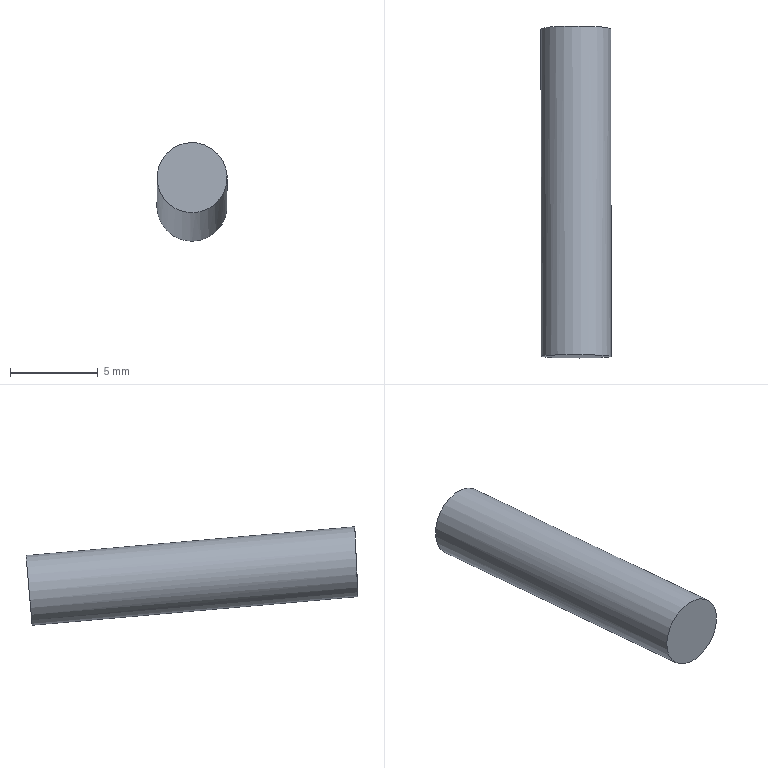Part | NX | features solid 2 | 1 solid | 3 faces | box 4 x 18.94 x 5.626 mm | volume 235.567 mm3 | plane 2 | cylinder 1 | commonest cylinder face diameters 4 x1
STEP:
#1=CARTESIAN_POINT('',(210.727,-28.358,-50.826));
#2=VERTEX_POINT('',#1);
#3=CARTESIAN_POINT('',(210.727,-28.184,-48.834));
#4=DIRECTION('',(0.,-0.9962,0.08716));
#5=DIRECTION('',(0.,-0.08716,-0.9962));
#6=AXIS2_PLACEMENT_3D('',#3,#4,#5);
#7=CIRCLE('',#6,2.);
#8=EDGE_CURVE('',#2,#2,#7,.T.);
#9=ORIENTED_EDGE('',*,*,#8,.F.);
#10=EDGE_LOOP('',(#9));
#11=FACE_BOUND('',#10,.T.);
#12=CARTESIAN_POINT('',(210.727,-28.184,-48.834));
#13=DIRECTION('',(0.,0.9962,-0.08716));
#14=DIRECTION('',(0.,0.08716,0.9962));
#15=AXIS2_PLACEMENT_3D('',#12,#13,#14);
#16=PLANE('',#15);
#17=ADVANCED_FACE('',(#11),#16,.T.);
#18=CARTESIAN_POINT('',(210.633,-46.949,-49.197));
#19=VERTEX_POINT('',#18);
#20=CARTESIAN_POINT('',(210.727,-46.858,-47.2));
#21=DIRECTION('',(0.001957,0.999,-0.04546));
#22=DIRECTION('',(-0.04675,-0.04532,-0.9979));
#23=AXIS2_PLACEMENT_3D('',#20,#21,#22);
#24=ELLIPSE('',#23,2.002,2.);
#25=EDGE_CURVE('',#19,#19,#24,.T.);
#26=ORIENTED_EDGE('',*,*,#25,.F.);
#27=EDGE_LOOP('',(#26));
#28=FACE_BOUND('',#27,.T.);
#29=CARTESIAN_POINT('',(128.811,-48.589,-88.763));
#30=DIRECTION('',(0.001957,0.999,-0.04546));
#31=DIRECTION('',(0.06617,0.04523,0.9968));
#32=AXIS2_PLACEMENT_3D('',#29,#30,#31);
#33=PLANE('',#32);
#34=ADVANCED_FACE('',(#28),#33,.F.);
#35=ORIENTED_EDGE('',*,*,#8,.T.);
#36=EDGE_LOOP('',(#35));
#37=FACE_BOUND('',#36,.T.);
#38=ORIENTED_EDGE('',*,*,#25,.T.);
#39=EDGE_LOOP('',(#38));
#40=FACE_BOUND('',#39,.T.);
#41=CARTESIAN_POINT('',(210.727,-48.107,-47.091));
#42=DIRECTION('',(0.,0.9962,-0.08716));
#43=DIRECTION('',(0.,0.08716,0.9962));
#44=AXIS2_PLACEMENT_3D('',#41,#42,#43);
#45=CYLINDRICAL_SURFACE('',#44,2.);
#46=ADVANCED_FACE('',(#37,#40),#45,.T.);
#47=CLOSED_SHELL('',(#17,#34,#46));
#48=MANIFOLD_SOLID_BREP('',#47);
#49=(LENGTH_UNIT()NAMED_UNIT(*)SI_UNIT(.MILLI.,.METRE.));
#50=UNCERTAINTY_MEASURE_WITH_UNIT(LENGTH_MEASURE(0.00001),#49,'','');
#51=(NAMED_UNIT(*)PLANE_ANGLE_UNIT()SI_UNIT($,.RADIAN.));
#52=(NAMED_UNIT(*)SI_UNIT($,.STERADIAN.)SOLID_ANGLE_UNIT());
#53=(GEOMETRIC_REPRESENTATION_CONTEXT(3)GLOBAL_UNCERTAINTY_ASSIGNED_CONTEXT((#50))GLOBAL_UNIT_ASSIGNED_CONTEXT((#49,#51,#52))REPRESENTATION_CONTEXT('',''));
#54=ADVANCED_BREP_SHAPE_REPRESENTATION('',(#48),#53);